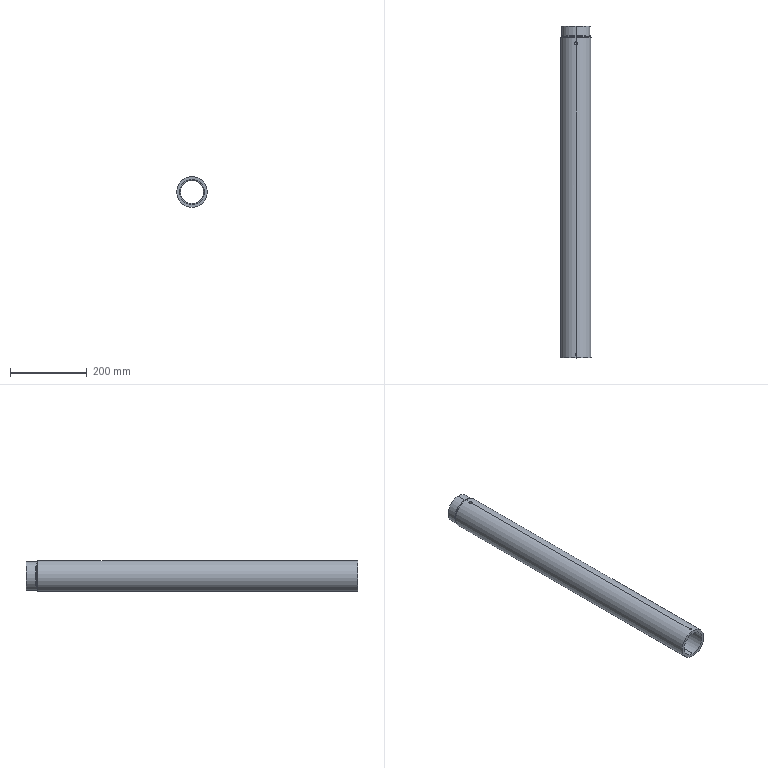Part | SolidWorks | features ICE 5, Chamfer 2, Extrusion 1, HoleWzd 1 | 1 solid | 24 faces | box 80 x 864.5 x 80 mm | volume 1857047 mm3 | cylinder 16 | plane 6 | cone 2 | commonest cylinder face diameters 4.2 x2 8 x2 60 x2 65 x2 73 x2 75 x2
STEP:
#1=CARTESIAN_POINT('',(0.,815.5,30.));
#2=VERTEX_POINT('',#1);
#3=CARTESIAN_POINT('',(-4.,819.5,29.732));
#4=VERTEX_POINT('',#3);
#5=CARTESIAN_POINT('',(0.,815.5,30.));
#6=CARTESIAN_POINT('',(-0.2612,815.5,30.));
#7=CARTESIAN_POINT('',(-0.5265,815.526,29.996));
#8=CARTESIAN_POINT('',(-1.04,815.629,29.983));
#9=CARTESIAN_POINT('',(-1.289,815.704,29.973));
#10=CARTESIAN_POINT('',(-1.773,815.905,29.949));
#11=CARTESIAN_POINT('',(-2.007,816.03,29.934));
#12=CARTESIAN_POINT('',(-2.44,816.32,29.901));
#13=CARTESIAN_POINT('',(-2.642,816.485,29.884));
#14=CARTESIAN_POINT('',(-3.015,816.858,29.849));
#15=CARTESIAN_POINT('',(-3.18,817.06,29.831));
#16=CARTESIAN_POINT('',(-3.47,817.493,29.799));
#17=CARTESIAN_POINT('',(-3.595,817.727,29.784));
#18=CARTESIAN_POINT('',(-3.796,818.211,29.759));
#19=CARTESIAN_POINT('',(-3.871,818.46,29.749));
#20=CARTESIAN_POINT('',(-3.974,818.974,29.736));
#21=CARTESIAN_POINT('',(-4.,819.239,29.732));
#22=CARTESIAN_POINT('',(-4.,819.5,29.732));
#23=B_SPLINE_CURVE_WITH_KNOTS('',3,(#5,#6,#7,#8,#9,#10,#11,#12,#13,#14,#15,#16,#17,#18,#19,#20,#21,#22),.UNSPECIFIED.,.F.,.F.,(4,2,2,2,2,2,2,2,4),(0.006261,0.007044,0.007826,0.008608,0.009391,0.01017,0.01096,0.01174,0.01252),.UNSPECIFIED.);
#24=EDGE_CURVE('',#2,#4,#23,.T.);
#25=ORIENTED_EDGE('',*,*,#24,.T.);
#26=CARTESIAN_POINT('',(-4.,819.5,39.799));
#27=VERTEX_POINT('',#26);
#28=CARTESIAN_POINT('',(-4.,819.5,10.));
#29=DIRECTION('',(0.,0.,1.));
#30=VECTOR('',#29,1000.);
#31=LINE('',#28,#30);
#32=EDGE_CURVE('',#4,#27,#31,.T.);
#33=ORIENTED_EDGE('',*,*,#32,.T.);
#34=CARTESIAN_POINT('',(0.,815.5,40.));
#35=VERTEX_POINT('',#34);
#36=CARTESIAN_POINT('',(0.,815.5,40.));
#37=CARTESIAN_POINT('',(-0.261,815.5,40.));
#38=CARTESIAN_POINT('',(-0.5262,815.526,39.997));
#39=CARTESIAN_POINT('',(-1.039,815.628,39.987));
#40=CARTESIAN_POINT('',(-1.289,815.704,39.98));
#41=CARTESIAN_POINT('',(-1.773,815.905,39.961));
#42=CARTESIAN_POINT('',(-2.007,816.03,39.95));
#43=CARTESIAN_POINT('',(-2.44,816.32,39.926));
#44=CARTESIAN_POINT('',(-2.642,816.485,39.913));
#45=CARTESIAN_POINT('',(-3.015,816.858,39.887));
#46=CARTESIAN_POINT('',(-3.181,817.06,39.874));
#47=CARTESIAN_POINT('',(-3.47,817.493,39.849));
#48=CARTESIAN_POINT('',(-3.595,817.727,39.838));
#49=CARTESIAN_POINT('',(-3.796,818.212,39.82));
#50=CARTESIAN_POINT('',(-3.872,818.461,39.812));
#51=CARTESIAN_POINT('',(-3.974,818.974,39.802));
#52=CARTESIAN_POINT('',(-4.,819.239,39.799));
#53=CARTESIAN_POINT('',(-4.,819.5,39.799));
#54=B_SPLINE_CURVE_WITH_KNOTS('',3,(#36,#37,#38,#39,#40,#41,#42,#43,#44,#45,#46,#47,#48,#49,#50,#51,#52,#53),.UNSPECIFIED.,.F.,.F.,(4,2,2,2,2,2,2,2,4),(0.006258,0.00704,0.007822,0.008604,0.009386,0.01017,0.01095,0.01173,0.01251),.UNSPECIFIED.);
#55=EDGE_CURVE('',#35,#27,#54,.T.);
#56=ORIENTED_EDGE('',*,*,#55,.F.);
#57=CARTESIAN_POINT('',(4.,819.5,39.799));
#58=VERTEX_POINT('',#57);
#59=CARTESIAN_POINT('',(4.,819.5,39.799));
#60=CARTESIAN_POINT('',(4.,819.235,39.799));
#61=CARTESIAN_POINT('',(3.974,818.975,39.802));
#62=CARTESIAN_POINT('',(3.872,818.464,39.812));
#63=CARTESIAN_POINT('',(3.795,818.21,39.82));
#64=CARTESIAN_POINT('',(3.594,817.725,39.838));
#65=CARTESIAN_POINT('',(3.471,817.495,39.849));
#66=CARTESIAN_POINT('',(3.181,817.061,39.874));
#67=CARTESIAN_POINT('',(3.012,816.855,39.887));
#68=CARTESIAN_POINT('',(2.643,816.486,39.913));
#69=CARTESIAN_POINT('',(2.441,816.321,39.926));
#70=CARTESIAN_POINT('',(2.004,816.028,39.95));
#71=CARTESIAN_POINT('',(1.771,815.904,39.961));
#72=CARTESIAN_POINT('',(1.29,815.705,39.98));
#73=CARTESIAN_POINT('',(1.037,815.628,39.987));
#74=CARTESIAN_POINT('',(0.5209,815.525,39.997));
#75=CARTESIAN_POINT('',(0.2611,815.5,40.));
#76=CARTESIAN_POINT('',(0.,815.5,40.));
#77=B_SPLINE_CURVE_WITH_KNOTS('',3,(#59,#60,#61,#62,#63,#64,#65,#66,#67,#68,#69,#70,#71,#72,#73,#74,#75,#76),.UNSPECIFIED.,.F.,.F.,(4,2,2,2,2,2,2,2,4),(0.,0.0007823,0.001565,0.002347,0.003129,0.003911,0.004694,0.005476,0.006258),.UNSPECIFIED.);
#78=EDGE_CURVE('',#58,#35,#77,.T.);
#79=ORIENTED_EDGE('',*,*,#78,.F.);
#80=CARTESIAN_POINT('',(4.,819.5,29.732));
#81=VERTEX_POINT('',#80);
#82=CARTESIAN_POINT('',(4.,819.5,10.));
#83=DIRECTION('',(0.,0.,1.));
#84=VECTOR('',#83,1000.);
#85=LINE('',#82,#84);
#86=EDGE_CURVE('',#81,#58,#85,.T.);
#87=ORIENTED_EDGE('',*,*,#86,.F.);
#88=CARTESIAN_POINT('',(4.,819.5,29.732));
#89=CARTESIAN_POINT('',(4.,819.235,29.732));
#90=CARTESIAN_POINT('',(3.974,818.975,29.736));
#91=CARTESIAN_POINT('',(3.872,818.463,29.749));
#92=CARTESIAN_POINT('',(3.795,818.209,29.759));
#93=CARTESIAN_POINT('',(3.594,817.725,29.784));
#94=CARTESIAN_POINT('',(3.471,817.495,29.799));
#95=CARTESIAN_POINT('',(3.181,817.06,29.831));
#96=CARTESIAN_POINT('',(3.012,816.855,29.849));
#97=CARTESIAN_POINT('',(2.643,816.486,29.884));
#98=CARTESIAN_POINT('',(2.442,816.321,29.901));
#99=CARTESIAN_POINT('',(2.004,816.028,29.934));
#100=CARTESIAN_POINT('',(1.772,815.904,29.949));
#101=CARTESIAN_POINT('',(1.29,815.705,29.973));
#102=CARTESIAN_POINT('',(1.038,815.628,29.983));
#103=CARTESIAN_POINT('',(0.5211,815.525,29.997));
#104=CARTESIAN_POINT('',(0.2613,815.5,30.));
#105=CARTESIAN_POINT('',(0.,815.5,30.));
#106=B_SPLINE_CURVE_WITH_KNOTS('',3,(#88,#89,#90,#91,#92,#93,#94,#95,#96,#97,#98,#99,#100,#101,#102,#103,#104,#105),.UNSPECIFIED.,.F.,.F.,(4,2,2,2,2,2,2,2,4),(0.,0.0007827,0.001565,0.002348,0.003131,0.003913,0.004696,0.005479,0.006261),.UNSPECIFIED.);
#107=EDGE_CURVE('',#81,#2,#106,.T.);
#108=ORIENTED_EDGE('',*,*,#107,.T.);
#109=EDGE_LOOP('',(#25,#33,#56,#79,#87,#108));
#110=FACE_OUTER_BOUND('',#109,.T.);
#111=CARTESIAN_POINT('',(0.,819.5,10.));
#112=DIRECTION('',(0.,0.,1.));
#113=DIRECTION('',(1.,0.,0.));
#114=AXIS2_PLACEMENT_3D('',#111,#112,#113);
#115=CYLINDRICAL_SURFACE('',#114,4.);
#116=ADVANCED_FACE('',(#110),#115,.F.);
#117=CARTESIAN_POINT('',(-2.1,9.,32.432));
#118=VERTEX_POINT('',#117);
#119=CARTESIAN_POINT('',(0.,6.9,32.5));
#120=VERTEX_POINT('',#119);
#121=CARTESIAN_POINT('',(-2.1,9.,32.432));
#122=CARTESIAN_POINT('',(-2.1,8.726,32.432));
#123=CARTESIAN_POINT('',(-2.045,8.449,32.436));
#124=CARTESIAN_POINT('',(-1.836,7.944,32.448));
#125=CARTESIAN_POINT('',(-1.679,7.709,32.457));
#126=CARTESIAN_POINT('',(-1.389,7.419,32.47));
#127=CARTESIAN_POINT('',(-1.281,7.33,32.475));
#128=CARTESIAN_POINT('',(-1.052,7.177,32.483));
#129=CARTESIAN_POINT('',(-0.9315,7.113,32.487));
#130=CARTESIAN_POINT('',(-0.6773,7.007,32.493));
#131=CARTESIAN_POINT('',(-0.5437,6.967,32.496));
#132=CARTESIAN_POINT('',(-0.2751,6.914,32.499));
#133=CARTESIAN_POINT('',(-0.1387,6.9,32.5));
#134=CARTESIAN_POINT('',(0.,6.9,32.5));
#135=B_SPLINE_CURVE_WITH_KNOTS('',3,(#121,#122,#123,#124,#125,#126,#127,#128,#129,#130,#131,#132,#133,#134),.UNSPECIFIED.,.F.,.F.,(4,2,2,2,2,2,4),(0.006567,0.007388,0.00821,0.00862,0.009031,0.009441,0.009852),.UNSPECIFIED.);
#136=EDGE_CURVE('',#118,#120,#135,.T.);
#137=ORIENTED_EDGE('',*,*,#136,.F.);
#138=CARTESIAN_POINT('',(-2.1,9.,39.945));
#139=VERTEX_POINT('',#138);
#140=CARTESIAN_POINT('',(-2.1,9.,40.));
#141=DIRECTION('',(0.,0.,1.));
#142=VECTOR('',#141,1000.);
#143=LINE('',#140,#142);
#144=EDGE_CURVE('',#118,#139,#143,.T.);
#145=ORIENTED_EDGE('',*,*,#144,.T.);
#146=CARTESIAN_POINT('',(0.,6.9,40.));
#147=VERTEX_POINT('',#146);
#148=CARTESIAN_POINT('',(0.,6.9,40.));
#149=CARTESIAN_POINT('',(-0.137,6.9,40.));
#150=CARTESIAN_POINT('',(-0.2761,6.914,39.999));
#151=CARTESIAN_POINT('',(-0.5454,6.967,39.997));
#152=CARTESIAN_POINT('',(-0.6762,7.007,39.994));
#153=CARTESIAN_POINT('',(-0.9305,7.112,39.989));
#154=CARTESIAN_POINT('',(-1.053,7.178,39.986));
#155=CARTESIAN_POINT('',(-1.281,7.33,39.98));
#156=CARTESIAN_POINT('',(-1.387,7.417,39.976));
#157=CARTESIAN_POINT('',(-1.583,7.613,39.969));
#158=CARTESIAN_POINT('',(-1.67,7.719,39.965));
#159=CARTESIAN_POINT('',(-1.822,7.947,39.959));
#160=CARTESIAN_POINT('',(-1.888,8.069,39.955));
#161=CARTESIAN_POINT('',(-1.993,8.324,39.95));
#162=CARTESIAN_POINT('',(-2.033,8.455,39.948));
#163=CARTESIAN_POINT('',(-2.086,8.724,39.946));
#164=CARTESIAN_POINT('',(-2.1,8.863,39.945));
#165=CARTESIAN_POINT('',(-2.1,9.,39.945));
#166=B_SPLINE_CURVE_WITH_KNOTS('',3,(#148,#149,#150,#151,#152,#153,#154,#155,#156,#157,#158,#159,#160,#161,#162,#163,#164,#165),.UNSPECIFIED.,.F.,.F.,(4,2,2,2,2,2,2,2,4),(0.003284,0.003694,0.004105,0.004515,0.004925,0.005336,0.005746,0.006156,0.006567),.UNSPECIFIED.);
#167=EDGE_CURVE('',#147,#139,#166,.T.);
#168=ORIENTED_EDGE('',*,*,#167,.F.);
#169=CARTESIAN_POINT('',(2.1,9.,39.945));
#170=VERTEX_POINT('',#169);
#171=CARTESIAN_POINT('',(2.1,9.,39.945));
#172=CARTESIAN_POINT('',(2.1,8.861,39.945));
#173=CARTESIAN_POINT('',(2.086,8.725,39.946));
#174=CARTESIAN_POINT('',(2.033,8.456,39.948));
#175=CARTESIAN_POINT('',(1.993,8.323,39.95));
#176=CARTESIAN_POINT('',(1.887,8.068,39.955));
#177=CARTESIAN_POINT('',(1.823,7.948,39.959));
#178=CARTESIAN_POINT('',(1.67,7.719,39.965));
#179=CARTESIAN_POINT('',(1.581,7.611,39.969));
#180=CARTESIAN_POINT('',(1.291,7.321,39.98));
#181=CARTESIAN_POINT('',(1.056,7.164,39.987));
#182=CARTESIAN_POINT('',(0.5506,6.955,39.997));
#183=CARTESIAN_POINT('',(0.2741,6.9,40.));
#184=CARTESIAN_POINT('',(0.,6.9,40.));
#185=B_SPLINE_CURVE_WITH_KNOTS('',3,(#171,#172,#173,#174,#175,#176,#177,#178,#179,#180,#181,#182,#183,#184),.UNSPECIFIED.,.F.,.F.,(4,2,2,2,2,2,4),(0.,0.0004105,0.000821,0.001232,0.001642,0.002463,0.003284),.UNSPECIFIED.);
#186=EDGE_CURVE('',#170,#147,#185,.T.);
#187=ORIENTED_EDGE('',*,*,#186,.F.);
#188=CARTESIAN_POINT('',(2.1,9.,32.432));
#189=VERTEX_POINT('',#188);
#190=CARTESIAN_POINT('',(2.1,9.,40.));
#191=DIRECTION('',(0.,0.,1.));
#192=VECTOR('',#191,1000.);
#193=LINE('',#190,#192);
#194=EDGE_CURVE('',#189,#170,#193,.T.);
#195=ORIENTED_EDGE('',*,*,#194,.F.);
#196=CARTESIAN_POINT('',(0.,6.9,32.5));
#197=CARTESIAN_POINT('',(0.1385,6.9,32.5));
#198=CARTESIAN_POINT('',(0.2753,6.914,32.499));
#199=CARTESIAN_POINT('',(0.5435,6.967,32.496));
#200=CARTESIAN_POINT('',(0.6766,7.007,32.493));
#201=CARTESIAN_POINT('',(0.931,7.113,32.487));
#202=CARTESIAN_POINT('',(1.052,7.177,32.483));
#203=CARTESIAN_POINT('',(1.28,7.329,32.475));
#204=CARTESIAN_POINT('',(1.388,7.418,32.471));
#205=CARTESIAN_POINT('',(1.581,7.611,32.462));
#206=CARTESIAN_POINT('',(1.668,7.717,32.457));
#207=CARTESIAN_POINT('',(1.822,7.946,32.449));
#208=CARTESIAN_POINT('',(1.887,8.068,32.445));
#209=CARTESIAN_POINT('',(2.044,8.447,32.436));
#210=CARTESIAN_POINT('',(2.1,8.723,32.432));
#211=CARTESIAN_POINT('',(2.1,9.,32.432));
#212=B_SPLINE_CURVE_WITH_KNOTS('',3,(#196,#197,#198,#199,#200,#201,#202,#203,#204,#205,#206,#207,#208,#209,#210,#211),.UNSPECIFIED.,.F.,.F.,(4,2,2,2,2,2,2,4),(0.009852,0.01026,0.01067,0.01108,0.01149,0.0119,0.01231,0.01313),.UNSPECIFIED.);
#213=EDGE_CURVE('',#120,#189,#212,.T.);
#214=ORIENTED_EDGE('',*,*,#213,.F.);
#215=EDGE_LOOP('',(#137,#145,#168,#187,#195,#214));
#216=FACE_OUTER_BOUND('',#215,.T.);
#217=CARTESIAN_POINT('',(0.,9.,40.));
#218=DIRECTION('',(0.,0.,1.));
#219=DIRECTION('',(1.,0.,0.));
#220=AXIS2_PLACEMENT_3D('',#217,#218,#219);
#221=CYLINDRICAL_SURFACE('',#220,2.1);
#222=ADVANCED_FACE('',(#216),#221,.F.);
#223=CARTESIAN_POINT('',(0.,51.5,30.));
#224=VERTEX_POINT('',#223);
#225=CARTESIAN_POINT('',(0.,51.5,-30.));
#226=VERTEX_POINT('',#225);
#227=CARTESIAN_POINT('',(0.,51.5,0.));
#228=DIRECTION('',(0.,-1.,0.));
#229=DIRECTION('',(0.,0.,-1.));
#230=AXIS2_PLACEMENT_3D('',#227,#228,#229);
#231=CIRCLE('',#230,30.);
#232=EDGE_CURVE('',#224,#226,#231,.T.);
#233=ORIENTED_EDGE('',*,*,#232,.F.);
#234=CARTESIAN_POINT('',(0.,50.,31.5));
#235=VERTEX_POINT('',#234);
#236=CARTESIAN_POINT('',(0.,51.5,30.));
#237=DIRECTION('',(0.,-0.7071,0.7071));
#238=VECTOR('',#237,1000.);
#239=LINE('',#236,#238);
#240=EDGE_CURVE('',#224,#235,#239,.T.);
#241=ORIENTED_EDGE('',*,*,#240,.T.);
#242=CARTESIAN_POINT('',(0.,50.,-31.5));
#243=VERTEX_POINT('',#242);
#244=CARTESIAN_POINT('',(0.,50.,0.));
#245=DIRECTION('',(0.,1.,0.));
#246=DIRECTION('',(0.,0.,-1.));
#247=AXIS2_PLACEMENT_3D('',#244,#245,#246);
#248=CIRCLE('',#247,31.5);
#249=EDGE_CURVE('',#243,#235,#248,.T.);
#250=ORIENTED_EDGE('',*,*,#249,.F.);
#251=CARTESIAN_POINT('',(0.,51.5,-30.));
#252=DIRECTION('',(0.,-0.7071,-0.7071));
#253=VECTOR('',#252,1000.);
#254=LINE('',#251,#253);
#255=EDGE_CURVE('',#226,#243,#254,.T.);
#256=ORIENTED_EDGE('',*,*,#255,.F.);
#257=EDGE_LOOP('',(#233,#241,#250,#256));
#258=FACE_OUTER_BOUND('',#257,.T.);
#259=CARTESIAN_POINT('',(0.,51.5,0.));
#260=DIRECTION('',(0.,-1.,0.));
#261=DIRECTION('',(0.,0.,-1.));
#262=AXIS2_PLACEMENT_3D('',#259,#260,#261);
#263=CONICAL_SURFACE('',#262,30.,0.7854);
#264=ADVANCED_FACE('',(#258),#263,.F.);
#265=CARTESIAN_POINT('',(0.,50.,32.5));
#266=VERTEX_POINT('',#265);
#267=CARTESIAN_POINT('',(0.,50.,-32.5));
#268=VERTEX_POINT('',#267);
#269=CARTESIAN_POINT('',(0.,50.,0.));
#270=DIRECTION('',(0.,-1.,0.));
#271=DIRECTION('',(0.,0.,-1.));
#272=AXIS2_PLACEMENT_3D('',#269,#270,#271);
#273=CIRCLE('',#272,32.5);
#274=EDGE_CURVE('',#266,#268,#273,.T.);
#275=ORIENTED_EDGE('',*,*,#274,.F.);
#276=CARTESIAN_POINT('',(0.,11.1,32.5));
#277=VERTEX_POINT('',#276);
#278=CARTESIAN_POINT('',(0.,50.,32.5));
#279=DIRECTION('',(0.,-1.,0.));
#280=VECTOR('',#279,1000.);
#281=LINE('',#278,#280);
#282=EDGE_CURVE('',#266,#277,#281,.T.);
#283=ORIENTED_EDGE('',*,*,#282,.T.);
#284=CARTESIAN_POINT('',(0.,11.1,32.5));
#285=CARTESIAN_POINT('',(-0.137,11.1,32.5));
#286=CARTESIAN_POINT('',(-0.2761,11.086,32.499));
#287=CARTESIAN_POINT('',(-0.5454,11.033,32.496));
#288=CARTESIAN_POINT('',(-0.6763,10.993,32.493));
#289=CARTESIAN_POINT('',(-0.9305,10.888,32.487));
#290=CARTESIAN_POINT('',(-1.053,10.822,32.483));
#291=CARTESIAN_POINT('',(-1.281,10.67,32.475));
#292=CARTESIAN_POINT('',(-1.387,10.583,32.471));
#293=CARTESIAN_POINT('',(-1.583,10.387,32.462));
#294=CARTESIAN_POINT('',(-1.67,10.281,32.457));
#295=CARTESIAN_POINT('',(-1.822,10.053,32.449));
#296=CARTESIAN_POINT('',(-1.888,9.931,32.445));
#297=CARTESIAN_POINT('',(-1.993,9.676,32.439));
#298=CARTESIAN_POINT('',(-2.033,9.545,32.436));
#299=CARTESIAN_POINT('',(-2.086,9.276,32.433));
#300=CARTESIAN_POINT('',(-2.1,9.137,32.432));
#301=CARTESIAN_POINT('',(-2.1,9.,32.432));
#302=B_SPLINE_CURVE_WITH_KNOTS('',3,(#284,#285,#286,#287,#288,#289,#290,#291,#292,#293,#294,#295,#296,#297,#298,#299,#300,#301),.UNSPECIFIED.,.F.,.F.,(4,2,2,2,2,2,2,2,4),(0.003284,0.003695,0.004105,0.004515,0.004926,0.005336,0.005747,0.006157,0.006567),.UNSPECIFIED.);
#303=EDGE_CURVE('',#277,#118,#302,.T.);
#304=ORIENTED_EDGE('',*,*,#303,.T.);
#305=ORIENTED_EDGE('',*,*,#136,.T.);
#306=CARTESIAN_POINT('',(0.,0.,32.5));
#307=VERTEX_POINT('',#306);
#308=CARTESIAN_POINT('',(0.,50.,32.5));
#309=DIRECTION('',(0.,-1.,0.));
#310=VECTOR('',#309,1000.);
#311=LINE('',#308,#310);
#312=EDGE_CURVE('',#120,#307,#311,.T.);
#313=ORIENTED_EDGE('',*,*,#312,.T.);
#314=CARTESIAN_POINT('',(0.,0.,-32.5));
#315=VERTEX_POINT('',#314);
#316=CARTESIAN_POINT('',(0.,0.,0.));
#317=DIRECTION('',(0.,-1.,0.));
#318=DIRECTION('',(0.,0.,-1.));
#319=AXIS2_PLACEMENT_3D('',#316,#317,#318);
#320=CIRCLE('',#319,32.5);
#321=EDGE_CURVE('',#307,#315,#320,.T.);
#322=ORIENTED_EDGE('',*,*,#321,.T.);
#323=CARTESIAN_POINT('',(0.,50.,-32.5));
#324=DIRECTION('',(0.,-1.,0.));
#325=VECTOR('',#324,1000.);
#326=LINE('',#323,#325);
#327=EDGE_CURVE('',#268,#315,#326,.T.);
#328=ORIENTED_EDGE('',*,*,#327,.F.);
#329=EDGE_LOOP('',(#275,#283,#304,#305,#313,#322,#328));
#330=FACE_OUTER_BOUND('',#329,.T.);
#331=CARTESIAN_POINT('',(0.,50.,0.));
#332=DIRECTION('',(0.,-1.,0.));
#333=DIRECTION('',(0.,0.,-1.));
#334=AXIS2_PLACEMENT_3D('',#331,#332,#333);
#335=CYLINDRICAL_SURFACE('',#334,32.5);
#336=ADVANCED_FACE('',(#330),#335,.F.);
#337=CARTESIAN_POINT('',(0.,834.5,38.));
#338=VERTEX_POINT('',#337);
#339=CARTESIAN_POINT('',(0.,834.5,-38.));
#340=VERTEX_POINT('',#339);
#341=CARTESIAN_POINT('',(0.,834.5,0.));
#342=DIRECTION('',(0.,1.,0.));
#343=DIRECTION('',(0.,0.,1.));
#344=AXIS2_PLACEMENT_3D('',#341,#342,#343);
#345=CIRCLE('',#344,38.);
#346=EDGE_CURVE('',#338,#340,#345,.T.);
#347=ORIENTED_EDGE('',*,*,#346,.T.);
#348=CARTESIAN_POINT('',(0.,836.5,-38.));
#349=VERTEX_POINT('',#348);
#350=CARTESIAN_POINT('',(0.,834.5,-38.));
#351=DIRECTION('',(0.,1.,0.));
#352=VECTOR('',#351,1000.);
#353=LINE('',#350,#352);
#354=EDGE_CURVE('',#340,#349,#353,.T.);
#355=ORIENTED_EDGE('',*,*,#354,.T.);
#356=CARTESIAN_POINT('',(0.,836.5,38.));
#357=VERTEX_POINT('',#356);
#358=CARTESIAN_POINT('',(0.,836.5,0.));
#359=DIRECTION('',(0.,1.,0.));
#360=DIRECTION('',(0.,0.,1.));
#361=AXIS2_PLACEMENT_3D('',#358,#359,#360);
#362=CIRCLE('',#361,38.);
#363=EDGE_CURVE('',#357,#349,#362,.T.);
#364=ORIENTED_EDGE('',*,*,#363,.F.);
#365=CARTESIAN_POINT('',(0.,834.5,38.));
#366=DIRECTION('',(0.,1.,0.));
#367=VECTOR('',#366,1000.);
#368=LINE('',#365,#367);
#369=EDGE_CURVE('',#338,#357,#368,.T.);
#370=ORIENTED_EDGE('',*,*,#369,.F.);
#371=EDGE_LOOP('',(#347,#355,#364,#370));
#372=FACE_OUTER_BOUND('',#371,.T.);
#373=CARTESIAN_POINT('',(0.,834.5,0.));
#374=DIRECTION('',(0.,1.,0.));
#375=DIRECTION('',(0.,0.,1.));
#376=AXIS2_PLACEMENT_3D('',#373,#374,#375);
#377=CYLINDRICAL_SURFACE('',#376,38.);
#378=ADVANCED_FACE('',(#372),#377,.T.);
#379=CARTESIAN_POINT('',(0.,836.5,36.5));
#380=VERTEX_POINT('',#379);
#381=CARTESIAN_POINT('',(0.,836.5,-36.5));
#382=VERTEX_POINT('',#381);
#383=CARTESIAN_POINT('',(0.,836.5,0.));
#384=DIRECTION('',(0.,1.,0.));
#385=DIRECTION('',(0.,0.,1.));
#386=AXIS2_PLACEMENT_3D('',#383,#384,#385);
#387=CIRCLE('',#386,36.5);
#388=EDGE_CURVE('',#380,#382,#387,.T.);
#389=ORIENTED_EDGE('',*,*,#388,.T.);
#390=CARTESIAN_POINT('',(0.,839.5,-36.5));
#391=VERTEX_POINT('',#390);
#392=CARTESIAN_POINT('',(0.,836.5,-36.5));
#393=DIRECTION('',(0.,1.,0.));
#394=VECTOR('',#393,1000.);
#395=LINE('',#392,#394);
#396=EDGE_CURVE('',#382,#391,#395,.T.);
#397=ORIENTED_EDGE('',*,*,#396,.T.);
#398=CARTESIAN_POINT('',(0.,839.5,36.5));
#399=VERTEX_POINT('',#398);
#400=CARTESIAN_POINT('',(0.,839.5,0.));
#401=DIRECTION('',(0.,1.,0.));
#402=DIRECTION('',(0.,0.,1.));
#403=AXIS2_PLACEMENT_3D('',#400,#401,#402);
#404=CIRCLE('',#403,36.5);
#405=EDGE_CURVE('',#399,#391,#404,.T.);
#406=ORIENTED_EDGE('',*,*,#405,.F.);
#407=CARTESIAN_POINT('',(0.,836.5,36.5));
#408=DIRECTION('',(0.,1.,0.));
#409=VECTOR('',#408,1000.);
#410=LINE('',#407,#409);
#411=EDGE_CURVE('',#380,#399,#410,.T.);
#412=ORIENTED_EDGE('',*,*,#411,.F.);
#413=EDGE_LOOP('',(#389,#397,#406,#412));
#414=FACE_OUTER_BOUND('',#413,.T.);
#415=CARTESIAN_POINT('',(0.,836.5,0.));
#416=DIRECTION('',(0.,1.,0.));
#417=DIRECTION('',(0.,0.,1.));
#418=AXIS2_PLACEMENT_3D('',#415,#416,#417);
#419=CYLINDRICAL_SURFACE('',#418,36.5);
#420=ADVANCED_FACE('',(#414),#419,.T.);
#421=CARTESIAN_POINT('',(0.,839.5,-37.5));
#422=VERTEX_POINT('',#421);
#423=CARTESIAN_POINT('',(0.,839.5,37.5));
#424=VERTEX_POINT('',#423);
#425=CARTESIAN_POINT('',(0.,839.5,0.));
#426=DIRECTION('',(0.,-1.,0.));
#427=DIRECTION('',(0.,0.,1.));
#428=AXIS2_PLACEMENT_3D('',#425,#426,#427);
#429=CIRCLE('',#428,37.5);
#430=EDGE_CURVE('',#422,#424,#429,.T.);
#431=ORIENTED_EDGE('',*,*,#430,.F.);
#432=CARTESIAN_POINT('',(0.,864.5,-37.5));
#433=VERTEX_POINT('',#432);
#434=CARTESIAN_POINT('',(0.,839.5,-37.5));
#435=DIRECTION('',(0.,1.,0.));
#436=VECTOR('',#435,1000.);
#437=LINE('',#434,#436);
#438=EDGE_CURVE('',#422,#433,#437,.T.);
#439=ORIENTED_EDGE('',*,*,#438,.T.);
#440=CARTESIAN_POINT('',(0.,864.5,37.5));
#441=VERTEX_POINT('',#440);
#442=CARTESIAN_POINT('',(0.,864.5,0.));
#443=DIRECTION('',(0.,1.,0.));
#444=DIRECTION('',(0.,0.,1.));
#445=AXIS2_PLACEMENT_3D('',#442,#443,#444);
#446=CIRCLE('',#445,37.5);
#447=EDGE_CURVE('',#441,#433,#446,.T.);
#448=ORIENTED_EDGE('',*,*,#447,.F.);
#449=CARTESIAN_POINT('',(0.,839.5,37.5));
#450=DIRECTION('',(0.,1.,0.));
#451=VECTOR('',#450,1000.);
#452=LINE('',#449,#451);
#453=EDGE_CURVE('',#424,#441,#452,.T.);
#454=ORIENTED_EDGE('',*,*,#453,.F.);
#455=EDGE_LOOP('',(#431,#439,#448,#454));
#456=FACE_OUTER_BOUND('',#455,.T.);
#457=CARTESIAN_POINT('',(0.,839.5,0.));
#458=DIRECTION('',(0.,1.,0.));
#459=DIRECTION('',(0.,0.,1.));
#460=AXIS2_PLACEMENT_3D('',#457,#458,#459);
#461=CYLINDRICAL_SURFACE('',#460,37.5);
#462=ADVANCED_FACE('',(#456),#461,.T.);
#463=CARTESIAN_POINT('',(0.,834.5,40.));
#464=VERTEX_POINT('',#463);
#465=CARTESIAN_POINT('',(0.,834.5,-40.));
#466=VERTEX_POINT('',#465);
#467=CARTESIAN_POINT('',(0.,834.5,0.));
#468=DIRECTION('',(0.,1.,0.));
#469=DIRECTION('',(0.,0.,1.));
#470=AXIS2_PLACEMENT_3D('',#467,#468,#469);
#471=CIRCLE('',#470,40.);
#472=EDGE_CURVE('',#464,#466,#471,.T.);
#473=ORIENTED_EDGE('',*,*,#472,.F.);
#474=CARTESIAN_POINT('',(0.,823.5,40.));
#475=VERTEX_POINT('',#474);
#476=CARTESIAN_POINT('',(0.,864.5,40.));
#477=DIRECTION('',(0.,-1.,0.));
#478=VECTOR('',#477,1000.);
#479=LINE('',#476,#478);
#480=EDGE_CURVE('',#464,#475,#479,.T.);
#481=ORIENTED_EDGE('',*,*,#480,.T.);
#482=CARTESIAN_POINT('',(0.,823.5,40.));
#483=CARTESIAN_POINT('',(0.2641,823.5,40.));
#484=CARTESIAN_POINT('',(0.5243,823.474,39.997));
#485=CARTESIAN_POINT('',(1.035,823.372,39.987));
#486=CARTESIAN_POINT('',(1.289,823.296,39.98));
#487=CARTESIAN_POINT('',(1.774,823.095,39.961));
#488=CARTESIAN_POINT('',(2.003,822.972,39.95));
#489=CARTESIAN_POINT('',(2.438,822.682,39.926));
#490=CARTESIAN_POINT('',(2.643,822.514,39.913));
#491=CARTESIAN_POINT('',(3.012,822.145,39.887));
#492=CARTESIAN_POINT('',(3.177,821.944,39.874));
#493=CARTESIAN_POINT('',(3.47,821.507,39.849));
#494=CARTESIAN_POINT('',(3.594,821.275,39.838));
#495=CARTESIAN_POINT('',(3.794,820.794,39.82));
#496=CARTESIAN_POINT('',(3.871,820.543,39.812));
#497=CARTESIAN_POINT('',(3.974,820.026,39.802));
#498=CARTESIAN_POINT('',(4.,819.764,39.799));
#499=CARTESIAN_POINT('',(4.,819.5,39.799));
#500=B_SPLINE_CURVE_WITH_KNOTS('',3,(#482,#483,#484,#485,#486,#487,#488,#489,#490,#491,#492,#493,#494,#495,#496,#497,#498,#499),.UNSPECIFIED.,.F.,.F.,(4,2,2,2,2,2,2,2,4),(0.01877,0.01955,0.02034,0.02112,0.0219,0.02268,0.02346,0.02424,0.02502),.UNSPECIFIED.);
#501=EDGE_CURVE('',#475,#58,#500,.T.);
#502=ORIENTED_EDGE('',*,*,#501,.T.);
#503=ORIENTED_EDGE('',*,*,#78,.T.);
#504=CARTESIAN_POINT('',(0.,11.1,40.));
#505=VERTEX_POINT('',#504);
#506=CARTESIAN_POINT('',(0.,864.5,40.));
#507=DIRECTION('',(0.,-1.,0.));
#508=VECTOR('',#507,1000.);
#509=LINE('',#506,#508);
#510=EDGE_CURVE('',#35,#505,#509,.T.);
#511=ORIENTED_EDGE('',*,*,#510,.T.);
#512=CARTESIAN_POINT('',(0.,11.1,40.));
#513=CARTESIAN_POINT('',(0.1385,11.1,40.));
#514=CARTESIAN_POINT('',(0.2753,11.086,39.999));
#515=CARTESIAN_POINT('',(0.5435,11.033,39.997));
#516=CARTESIAN_POINT('',(0.6766,10.993,39.994));
#517=CARTESIAN_POINT('',(0.931,10.887,39.989));
#518=CARTESIAN_POINT('',(1.052,10.823,39.986));
#519=CARTESIAN_POINT('',(1.28,10.671,39.98));
#520=CARTESIAN_POINT('',(1.388,10.582,39.976));
#521=CARTESIAN_POINT('',(1.581,10.389,39.969));
#522=CARTESIAN_POINT('',(1.668,10.283,39.965));
#523=CARTESIAN_POINT('',(1.822,10.054,39.959));
#524=CARTESIAN_POINT('',(1.887,9.932,39.955));
#525=CARTESIAN_POINT('',(2.044,9.553,39.948));
#526=CARTESIAN_POINT('',(2.1,9.277,39.945));
#527=CARTESIAN_POINT('',(2.1,9.,39.945));
#528=B_SPLINE_CURVE_WITH_KNOTS('',3,(#512,#513,#514,#515,#516,#517,#518,#519,#520,#521,#522,#523,#524,#525,#526,#527),.UNSPECIFIED.,.F.,.F.,(4,2,2,2,2,2,2,4),(0.009851,0.01026,0.01067,0.01108,0.01149,0.0119,0.01231,0.01313),.UNSPECIFIED.);
#529=EDGE_CURVE('',#505,#170,#528,.T.);
#530=ORIENTED_EDGE('',*,*,#529,.T.);
#531=ORIENTED_EDGE('',*,*,#186,.T.);
#532=CARTESIAN_POINT('',(0.,0.,40.));
#533=VERTEX_POINT('',#532);
#534=CARTESIAN_POINT('',(0.,864.5,40.));
#535=DIRECTION('',(0.,-1.,0.));
#536=VECTOR('',#535,1000.);
#537=LINE('',#534,#536);
#538=EDGE_CURVE('',#147,#533,#537,.T.);
#539=ORIENTED_EDGE('',*,*,#538,.T.);
#540=CARTESIAN_POINT('',(0.,0.,-40.));
#541=VERTEX_POINT('',#540);
#542=CARTESIAN_POINT('',(0.,0.,0.));
#543=DIRECTION('',(0.,1.,0.));
#544=DIRECTION('',(0.,0.,1.));
#545=AXIS2_PLACEMENT_3D('',#542,#543,#544);
#546=CIRCLE('',#545,40.);
#547=EDGE_CURVE('',#533,#541,#546,.T.);
#548=ORIENTED_EDGE('',*,*,#547,.T.);
#549=CARTESIAN_POINT('',(0.,864.5,-40.));
#550=DIRECTION('',(0.,-1.,0.));
#551=VECTOR('',#550,1000.);
#552=LINE('',#549,#551);
#553=EDGE_CURVE('',#466,#541,#552,.T.);
#554=ORIENTED_EDGE('',*,*,#553,.F.);
#555=EDGE_LOOP('',(#473,#481,#502,#503,#511,#530,#531,#539,#548,#554));
#556=FACE_OUTER_BOUND('',#555,.T.);
#557=CARTESIAN_POINT('',(0.,864.5,0.));
#558=DIRECTION('',(0.,-1.,0.));
#559=DIRECTION('',(0.,0.,-1.));
#560=AXIS2_PLACEMENT_3D('',#557,#558,#559);
#561=CYLINDRICAL_SURFACE('',#560,40.);
#562=ADVANCED_FACE('',(#556),#561,.T.);
#563=CARTESIAN_POINT('',(0.,864.5,-30.));
#564=VERTEX_POINT('',#563);
#565=CARTESIAN_POINT('',(0.,864.5,30.));
#566=VERTEX_POINT('',#565);
#567=CARTESIAN_POINT('',(0.,864.5,0.));
#568=DIRECTION('',(0.,1.,0.));
#569=DIRECTION('',(0.,0.,1.));
#570=AXIS2_PLACEMENT_3D('',#567,#568,#569);
#571=CIRCLE('',#570,30.);
#572=EDGE_CURVE('',#564,#566,#571,.T.);
#573=ORIENTED_EDGE('',*,*,#572,.T.);
#574=CARTESIAN_POINT('',(0.,823.5,30.));
#575=VERTEX_POINT('',#574);
#576=CARTESIAN_POINT('',(0.,864.5,30.));
#577=DIRECTION('',(0.,-1.,0.));
#578=VECTOR('',#577,1000.);
#579=LINE('',#576,#578);
#580=EDGE_CURVE('',#566,#575,#579,.T.);
#581=ORIENTED_EDGE('',*,*,#580,.T.);
#582=CARTESIAN_POINT('',(-4.,819.5,29.732));
#583=CARTESIAN_POINT('',(-4.,819.761,29.732));
#584=CARTESIAN_POINT('',(-3.975,820.021,29.736));
#585=CARTESIAN_POINT('',(-3.872,820.538,29.749));
#586=CARTESIAN_POINT('',(-3.795,820.79,29.759));
#587=CARTESIAN_POINT('',(-3.596,821.272,29.784));
#588=CARTESIAN_POINT('',(-3.471,821.505,29.799));
#589=CARTESIAN_POINT('',(-3.179,821.942,29.831));
#590=CARTESIAN_POINT('',(-3.014,822.143,29.849));
#591=CARTESIAN_POINT('',(-2.645,822.512,29.884));
#592=CARTESIAN_POINT('',(-2.439,822.681,29.901));
#593=CARTESIAN_POINT('',(-2.005,822.971,29.934));
#594=CARTESIAN_POINT('',(-1.775,823.094,29.948));
#595=CARTESIAN_POINT('',(-1.291,823.295,29.973));
#596=CARTESIAN_POINT('',(-1.037,823.372,29.983));
#597=CARTESIAN_POINT('',(-0.525,823.474,29.996));
#598=CARTESIAN_POINT('',(-0.2645,823.5,30.));
#599=CARTESIAN_POINT('',(0.,823.5,30.));
#600=B_SPLINE_CURVE_WITH_KNOTS('',3,(#582,#583,#584,#585,#586,#587,#588,#589,#590,#591,#592,#593,#594,#595,#596,#597,#598,#599),.UNSPECIFIED.,.F.,.F.,(4,2,2,2,2,2,2,2,4),(0.01252,0.0133,0.01409,0.01487,0.01565,0.01643,0.01722,0.018,0.01878),.UNSPECIFIED.);
#601=EDGE_CURVE('',#4,#575,#600,.T.);
#602=ORIENTED_EDGE('',*,*,#601,.F.);
#603=ORIENTED_EDGE('',*,*,#24,.F.);
#604=CARTESIAN_POINT('',(0.,864.5,30.));
#605=DIRECTION('',(0.,-1.,0.));
#606=VECTOR('',#605,1000.);
#607=LINE('',#604,#606);
#608=EDGE_CURVE('',#2,#224,#607,.T.);
#609=ORIENTED_EDGE('',*,*,#608,.T.);
#610=ORIENTED_EDGE('',*,*,#232,.T.);
#611=CARTESIAN_POINT('',(0.,864.5,-30.));
#612=DIRECTION('',(0.,-1.,0.));
#613=VECTOR('',#612,1000.);
#614=LINE('',#611,#613);
#615=EDGE_CURVE('',#564,#226,#614,.T.);
#616=ORIENTED_EDGE('',*,*,#615,.F.);
#617=EDGE_LOOP('',(#573,#581,#602,#603,#609,#610,#616));
#618=FACE_OUTER_BOUND('',#617,.T.);
#619=CARTESIAN_POINT('',(0.,864.5,0.));
#620=DIRECTION('',(0.,-1.,0.));
#621=DIRECTION('',(0.,0.,-1.));
#622=AXIS2_PLACEMENT_3D('',#619,#620,#621);
#623=CYLINDRICAL_SURFACE('',#622,30.);
#624=ADVANCED_FACE('',(#618),#623,.F.);
#625=ORIENTED_EDGE('',*,*,#580,.F.);
#626=CARTESIAN_POINT('',(0.,864.5,0.));
#627=DIRECTION('',(0.,1.,0.));
#628=DIRECTION('',(0.,0.,1.));
#629=AXIS2_PLACEMENT_3D('',#626,#627,#628);
#630=CIRCLE('',#629,30.);
#631=EDGE_CURVE('',#566,#564,#630,.T.);
#632=ORIENTED_EDGE('',*,*,#631,.T.);
#633=ORIENTED_EDGE('',*,*,#615,.T.);
#634=CARTESIAN_POINT('',(0.,51.5,0.));
#635=DIRECTION('',(0.,-1.,0.));
#636=DIRECTION('',(0.,0.,-1.));
#637=AXIS2_PLACEMENT_3D('',#634,#635,#636);
#638=CIRCLE('',#637,30.);
#639=EDGE_CURVE('',#226,#224,#638,.T.);
#640=ORIENTED_EDGE('',*,*,#639,.T.);
#641=ORIENTED_EDGE('',*,*,#608,.F.);
#642=ORIENTED_EDGE('',*,*,#107,.F.);
#643=CARTESIAN_POINT('',(0.,823.5,30.));
#644=CARTESIAN_POINT('',(0.2643,823.5,30.));
#645=CARTESIAN_POINT('',(0.5242,823.474,29.997));
#646=CARTESIAN_POINT('',(1.036,823.372,29.983));
#647=CARTESIAN_POINT('',(1.29,823.295,29.973));
#648=CARTESIAN_POINT('',(1.774,823.095,29.949));
#649=CARTESIAN_POINT('',(2.003,822.972,29.934));
#650=CARTESIAN_POINT('',(2.438,822.682,29.902));
#651=CARTESIAN_POINT('',(2.643,822.513,29.884));
#652=CARTESIAN_POINT('',(3.012,822.145,29.849));
#653=CARTESIAN_POINT('',(3.177,821.944,29.832));
#654=CARTESIAN_POINT('',(3.47,821.507,29.799));
#655=CARTESIAN_POINT('',(3.594,821.275,29.784));
#656=CARTESIAN_POINT('',(3.794,820.795,29.759));
#657=CARTESIAN_POINT('',(3.871,820.543,29.749));
#658=CARTESIAN_POINT('',(3.974,820.026,29.736));
#659=CARTESIAN_POINT('',(4.,819.764,29.732));
#660=CARTESIAN_POINT('',(4.,819.5,29.732));
#661=B_SPLINE_CURVE_WITH_KNOTS('',3,(#643,#644,#645,#646,#647,#648,#649,#650,#651,#652,#653,#654,#655,#656,#657,#658,#659,#660),.UNSPECIFIED.,.F.,.F.,(4,2,2,2,2,2,2,2,4),(0.01878,0.01956,0.02034,0.02113,0.02191,0.02269,0.02347,0.02425,0.02504),.UNSPECIFIED.);
#662=EDGE_CURVE('',#575,#81,#661,.T.);
#663=ORIENTED_EDGE('',*,*,#662,.F.);
#664=EDGE_LOOP('',(#625,#632,#633,#640,#641,#642,#663));
#665=FACE_OUTER_BOUND('',#664,.T.);
#666=CARTESIAN_POINT('',(0.,864.5,0.));
#667=DIRECTION('',(0.,-1.,0.));
#668=DIRECTION('',(0.,0.,-1.));
#669=AXIS2_PLACEMENT_3D('',#666,#667,#668);
#670=CYLINDRICAL_SURFACE('',#669,30.);
#671=ADVANCED_FACE('',(#665),#670,.F.);
#672=ORIENTED_EDGE('',*,*,#480,.F.);
#673=CARTESIAN_POINT('',(0.,834.5,0.));
#674=DIRECTION('',(0.,1.,0.));
#675=DIRECTION('',(0.,0.,1.));
#676=AXIS2_PLACEMENT_3D('',#673,#674,#675);
#677=CIRCLE('',#676,40.);
#678=EDGE_CURVE('',#466,#464,#677,.T.);
#679=ORIENTED_EDGE('',*,*,#678,.F.);
#680=ORIENTED_EDGE('',*,*,#553,.T.);
#681=CARTESIAN_POINT('',(0.,0.,0.));
#682=DIRECTION('',(0.,1.,0.));
#683=DIRECTION('',(0.,0.,1.));
#684=AXIS2_PLACEMENT_3D('',#681,#682,#683);
#685=CIRCLE('',#684,40.);
#686=EDGE_CURVE('',#541,#533,#685,.T.);
#687=ORIENTED_EDGE('',*,*,#686,.T.);
#688=ORIENTED_EDGE('',*,*,#538,.F.);
#689=ORIENTED_EDGE('',*,*,#167,.T.);
#690=CARTESIAN_POINT('',(-2.1,9.,39.945));
#691=CARTESIAN_POINT('',(-2.1,9.137,39.945));
#692=CARTESIAN_POINT('',(-2.087,9.273,39.946));
#693=CARTESIAN_POINT('',(-2.033,9.544,39.948));
#694=CARTESIAN_POINT('',(-1.993,9.677,39.95));
#695=CARTESIAN_POINT('',(-1.836,10.056,39.958));
#696=CARTESIAN_POINT('',(-1.679,10.291,39.965));
#697=CARTESIAN_POINT('',(-1.389,10.581,39.976));
#698=CARTESIAN_POINT('',(-1.281,10.67,39.98));
#699=CARTESIAN_POINT('',(-1.052,10.823,39.986));
#700=CARTESIAN_POINT('',(-0.9314,10.887,39.989));
#701=CARTESIAN_POINT('',(-0.6772,10.993,39.994));
#702=CARTESIAN_POINT('',(-0.5436,11.033,39.997));
#703=CARTESIAN_POINT('',(-0.275,11.086,39.999));
#704=CARTESIAN_POINT('',(-0.1386,11.1,40.));
#705=CARTESIAN_POINT('',(0.,11.1,40.));
#706=B_SPLINE_CURVE_WITH_KNOTS('',3,(#690,#691,#692,#693,#694,#695,#696,#697,#698,#699,#700,#701,#702,#703,#704,#705),.UNSPECIFIED.,.F.,.F.,(4,2,2,2,2,2,2,4),(0.006567,0.006977,0.007388,0.008209,0.008619,0.00903,0.00944,0.009851),.UNSPECIFIED.);
#707=EDGE_CURVE('',#139,#505,#706,.T.);
#708=ORIENTED_EDGE('',*,*,#707,.T.);
#709=ORIENTED_EDGE('',*,*,#510,.F.);
#710=ORIENTED_EDGE('',*,*,#55,.T.);
#711=CARTESIAN_POINT('',(-4.,819.5,39.799));
#712=CARTESIAN_POINT('',(-4.,819.761,39.799));
#713=CARTESIAN_POINT('',(-3.975,820.021,39.802));
#714=CARTESIAN_POINT('',(-3.872,820.537,39.812));
#715=CARTESIAN_POINT('',(-3.795,820.79,39.82));
#716=CARTESIAN_POINT('',(-3.596,821.272,39.838));
#717=CARTESIAN_POINT('',(-3.472,821.504,39.849));
#718=CARTESIAN_POINT('',(-3.179,821.942,39.874));
#719=CARTESIAN_POINT('',(-3.014,822.143,39.887));
#720=CARTESIAN_POINT('',(-2.645,822.512,39.913));
#721=CARTESIAN_POINT('',(-2.439,822.681,39.926));
#722=CARTESIAN_POINT('',(-2.004,822.971,39.95));
#723=CARTESIAN_POINT('',(-1.775,823.094,39.961));
#724=CARTESIAN_POINT('',(-1.29,823.295,39.98));
#725=CARTESIAN_POINT('',(-1.036,823.372,39.987));
#726=CARTESIAN_POINT('',(-0.5244,823.474,39.997));
#727=CARTESIAN_POINT('',(-0.2644,823.5,40.));
#728=CARTESIAN_POINT('',(0.,823.5,40.));
#729=B_SPLINE_CURVE_WITH_KNOTS('',3,(#711,#712,#713,#714,#715,#716,#717,#718,#719,#720,#721,#722,#723,#724,#725,#726,#727,#728),.UNSPECIFIED.,.F.,.F.,(4,2,2,2,2,2,2,2,4),(0.01251,0.0133,0.01408,0.01486,0.01564,0.01643,0.01721,0.01799,0.01877),.UNSPECIFIED.);
#730=EDGE_CURVE('',#27,#475,#729,.T.);
#731=ORIENTED_EDGE('',*,*,#730,.T.);
#732=EDGE_LOOP('',(#672,#679,#680,#687,#688,#689,#708,#709,#710,#731));
#733=FACE_OUTER_BOUND('',#732,.T.);
#734=CARTESIAN_POINT('',(0.,864.5,0.));
#735=DIRECTION('',(0.,-1.,0.));
#736=DIRECTION('',(0.,0.,-1.));
#737=AXIS2_PLACEMENT_3D('',#734,#735,#736);
#738=CYLINDRICAL_SURFACE('',#737,40.);
#739=ADVANCED_FACE('',(#733),#738,.T.);
#740=ORIENTED_EDGE('',*,*,#388,.F.);
#741=CARTESIAN_POINT('',(0.,836.5,0.));
#742=DIRECTION('',(0.,1.,0.));
#743=DIRECTION('',(0.,0.,1.));
#744=AXIS2_PLACEMENT_3D('',#741,#742,#743);
#745=CIRCLE('',#744,36.5);
#746=EDGE_CURVE('',#382,#380,#745,.T.);
#747=ORIENTED_EDGE('',*,*,#746,.F.);
#748=EDGE_LOOP('',(#740,#747));
#749=FACE_BOUND('',#748,.T.);
#750=ORIENTED_EDGE('',*,*,#363,.T.);
#751=CARTESIAN_POINT('',(0.,836.5,0.));
#752=DIRECTION('',(0.,1.,0.));
#753=DIRECTION('',(0.,0.,1.));
#754=AXIS2_PLACEMENT_3D('',#751,#752,#753);
#755=CIRCLE('',#754,38.);
#756=EDGE_CURVE('',#349,#357,#755,.T.);
#757=ORIENTED_EDGE('',*,*,#756,.T.);
#758=EDGE_LOOP('',(#750,#757));
#759=FACE_OUTER_BOUND('',#758,.T.);
#760=CARTESIAN_POINT('',(0.,836.5,0.));
#761=DIRECTION('',(0.,1.,0.));
#762=DIRECTION('',(0.,0.,1.));
#763=AXIS2_PLACEMENT_3D('',#760,#761,#762);
#764=PLANE('',#763);
#765=ADVANCED_FACE('',(#749,#759),#764,.T.);
#766=ORIENTED_EDGE('',*,*,#572,.F.);
#767=ORIENTED_EDGE('',*,*,#631,.F.);
#768=EDGE_LOOP('',(#766,#767));
#769=FACE_BOUND('',#768,.T.);
#770=ORIENTED_EDGE('',*,*,#447,.T.);
#771=CARTESIAN_POINT('',(0.,864.5,0.));
#772=DIRECTION('',(0.,1.,0.));
#773=DIRECTION('',(0.,0.,1.));
#774=AXIS2_PLACEMENT_3D('',#771,#772,#773);
#775=CIRCLE('',#774,37.5);
#776=EDGE_CURVE('',#433,#441,#775,.T.);
#777=ORIENTED_EDGE('',*,*,#776,.T.);
#778=EDGE_LOOP('',(#770,#777));
#779=FACE_OUTER_BOUND('',#778,.T.);
#780=CARTESIAN_POINT('',(0.,864.5,0.));
#781=DIRECTION('',(0.,1.,0.));
#782=DIRECTION('',(0.,0.,1.));
#783=AXIS2_PLACEMENT_3D('',#780,#781,#782);
#784=PLANE('',#783);
#785=ADVANCED_FACE('',(#769,#779),#784,.T.);
#786=CARTESIAN_POINT('',(0.,0.,0.));
#787=DIRECTION('',(0.,-1.,0.));
#788=DIRECTION('',(0.,0.,-1.));
#789=AXIS2_PLACEMENT_3D('',#786,#787,#788);
#790=CIRCLE('',#789,32.5);
#791=EDGE_CURVE('',#315,#307,#790,.T.);
#792=ORIENTED_EDGE('',*,*,#791,.F.);
#793=ORIENTED_EDGE('',*,*,#321,.F.);
#794=EDGE_LOOP('',(#792,#793));
#795=FACE_BOUND('',#794,.T.);
#796=ORIENTED_EDGE('',*,*,#686,.F.);
#797=ORIENTED_EDGE('',*,*,#547,.F.);
#798=EDGE_LOOP('',(#796,#797));
#799=FACE_OUTER_BOUND('',#798,.T.);
#800=CARTESIAN_POINT('',(0.,0.,0.));
#801=DIRECTION('',(0.,1.,0.));
#802=DIRECTION('',(0.,0.,1.));
#803=AXIS2_PLACEMENT_3D('',#800,#801,#802);
#804=PLANE('',#803);
#805=ADVANCED_FACE('',(#795,#799),#804,.F.);
#806=ORIENTED_EDGE('',*,*,#438,.F.);
#807=CARTESIAN_POINT('',(0.,839.5,0.));
#808=DIRECTION('',(0.,-1.,0.));
#809=DIRECTION('',(0.,0.,1.));
#810=AXIS2_PLACEMENT_3D('',#807,#808,#809);
#811=CIRCLE('',#810,37.5);
#812=EDGE_CURVE('',#424,#422,#811,.T.);
#813=ORIENTED_EDGE('',*,*,#812,.F.);
#814=ORIENTED_EDGE('',*,*,#453,.T.);
#815=ORIENTED_EDGE('',*,*,#776,.F.);
#816=EDGE_LOOP('',(#806,#813,#814,#815));
#817=FACE_OUTER_BOUND('',#816,.T.);
#818=CARTESIAN_POINT('',(0.,839.5,0.));
#819=DIRECTION('',(0.,1.,0.));
#820=DIRECTION('',(0.,0.,1.));
#821=AXIS2_PLACEMENT_3D('',#818,#819,#820);
#822=CYLINDRICAL_SURFACE('',#821,37.5);
#823=ADVANCED_FACE('',(#817),#822,.T.);
#824=ORIENTED_EDGE('',*,*,#812,.T.);
#825=ORIENTED_EDGE('',*,*,#430,.T.);
#826=EDGE_LOOP('',(#824,#825));
#827=FACE_OUTER_BOUND('',#826,.T.);
#828=ORIENTED_EDGE('',*,*,#405,.T.);
#829=CARTESIAN_POINT('',(0.,839.5,0.));
#830=DIRECTION('',(0.,1.,0.));
#831=DIRECTION('',(0.,0.,1.));
#832=AXIS2_PLACEMENT_3D('',#829,#830,#831);
#833=CIRCLE('',#832,36.5);
#834=EDGE_CURVE('',#391,#399,#833,.T.);
#835=ORIENTED_EDGE('',*,*,#834,.T.);
#836=EDGE_LOOP('',(#828,#835));
#837=FACE_BOUND('',#836,.T.);
#838=CARTESIAN_POINT('',(0.,839.5,0.));
#839=DIRECTION('',(0.,1.,0.));
#840=DIRECTION('',(0.,0.,1.));
#841=AXIS2_PLACEMENT_3D('',#838,#839,#840);
#842=PLANE('',#841);
#843=ADVANCED_FACE('',(#827,#837),#842,.F.);
#844=ORIENTED_EDGE('',*,*,#396,.F.);
#845=ORIENTED_EDGE('',*,*,#746,.T.);
#846=ORIENTED_EDGE('',*,*,#411,.T.);
#847=ORIENTED_EDGE('',*,*,#834,.F.);
#848=EDGE_LOOP('',(#844,#845,#846,#847));
#849=FACE_OUTER_BOUND('',#848,.T.);
#850=CARTESIAN_POINT('',(0.,836.5,0.));
#851=DIRECTION('',(0.,1.,0.));
#852=DIRECTION('',(0.,0.,1.));
#853=AXIS2_PLACEMENT_3D('',#850,#851,#852);
#854=CYLINDRICAL_SURFACE('',#853,36.5);
#855=ADVANCED_FACE('',(#849),#854,.T.);
#856=ORIENTED_EDGE('',*,*,#346,.F.);
#857=CARTESIAN_POINT('',(0.,834.5,0.));
#858=DIRECTION('',(0.,1.,0.));
#859=DIRECTION('',(0.,0.,1.));
#860=AXIS2_PLACEMENT_3D('',#857,#858,#859);
#861=CIRCLE('',#860,38.);
#862=EDGE_CURVE('',#340,#338,#861,.T.);
#863=ORIENTED_EDGE('',*,*,#862,.F.);
#864=EDGE_LOOP('',(#856,#863));
#865=FACE_BOUND('',#864,.T.);
#866=ORIENTED_EDGE('',*,*,#678,.T.);
#867=ORIENTED_EDGE('',*,*,#472,.T.);
#868=EDGE_LOOP('',(#866,#867));
#869=FACE_OUTER_BOUND('',#868,.T.);
#870=CARTESIAN_POINT('',(0.,834.5,0.));
#871=DIRECTION('',(0.,1.,0.));
#872=DIRECTION('',(0.,0.,1.));
#873=AXIS2_PLACEMENT_3D('',#870,#871,#872);
#874=PLANE('',#873);
#875=ADVANCED_FACE('',(#865,#869),#874,.T.);
#876=ORIENTED_EDGE('',*,*,#354,.F.);
#877=ORIENTED_EDGE('',*,*,#862,.T.);
#878=ORIENTED_EDGE('',*,*,#369,.T.);
#879=ORIENTED_EDGE('',*,*,#756,.F.);
#880=EDGE_LOOP('',(#876,#877,#878,#879));
#881=FACE_OUTER_BOUND('',#880,.T.);
#882=CARTESIAN_POINT('',(0.,834.5,0.));
#883=DIRECTION('',(0.,1.,0.));
#884=DIRECTION('',(0.,0.,1.));
#885=AXIS2_PLACEMENT_3D('',#882,#883,#884);
#886=CYLINDRICAL_SURFACE('',#885,38.);
#887=ADVANCED_FACE('',(#881),#886,.T.);
#888=ORIENTED_EDGE('',*,*,#282,.F.);
#889=CARTESIAN_POINT('',(0.,50.,0.));
#890=DIRECTION('',(0.,-1.,0.));
#891=DIRECTION('',(0.,0.,-1.));
#892=AXIS2_PLACEMENT_3D('',#889,#890,#891);
#893=CIRCLE('',#892,32.5);
#894=EDGE_CURVE('',#268,#266,#893,.T.);
#895=ORIENTED_EDGE('',*,*,#894,.F.);
#896=ORIENTED_EDGE('',*,*,#327,.T.);
#897=ORIENTED_EDGE('',*,*,#791,.T.);
#898=ORIENTED_EDGE('',*,*,#312,.F.);
#899=ORIENTED_EDGE('',*,*,#213,.T.);
#900=CARTESIAN_POINT('',(2.1,9.,32.432));
#901=CARTESIAN_POINT('',(2.1,9.139,32.432));
#902=CARTESIAN_POINT('',(2.086,9.275,32.433));
#903=CARTESIAN_POINT('',(2.033,9.544,32.436));
#904=CARTESIAN_POINT('',(1.993,9.677,32.439));
#905=CARTESIAN_POINT('',(1.887,9.932,32.445));
#906=CARTESIAN_POINT('',(1.823,10.052,32.449));
#907=CARTESIAN_POINT('',(1.67,10.281,32.457));
#908=CARTESIAN_POINT('',(1.581,10.389,32.462));
#909=CARTESIAN_POINT('',(1.291,10.679,32.475));
#910=CARTESIAN_POINT('',(1.056,10.836,32.484));
#911=CARTESIAN_POINT('',(0.5506,11.045,32.496));
#912=CARTESIAN_POINT('',(0.2741,11.1,32.5));
#913=CARTESIAN_POINT('',(0.,11.1,32.5));
#914=B_SPLINE_CURVE_WITH_KNOTS('',3,(#900,#901,#902,#903,#904,#905,#906,#907,#908,#909,#910,#911,#912,#913),.UNSPECIFIED.,.F.,.F.,(4,2,2,2,2,2,4),(0.,0.0004105,0.0008211,0.001232,0.001642,0.002463,0.003284),.UNSPECIFIED.);
#915=EDGE_CURVE('',#189,#277,#914,.T.);
#916=ORIENTED_EDGE('',*,*,#915,.T.);
#917=EDGE_LOOP('',(#888,#895,#896,#897,#898,#899,#916));
#918=FACE_OUTER_BOUND('',#917,.T.);
#919=CARTESIAN_POINT('',(0.,50.,0.));
#920=DIRECTION('',(0.,-1.,0.));
#921=DIRECTION('',(0.,0.,-1.));
#922=AXIS2_PLACEMENT_3D('',#919,#920,#921);
#923=CYLINDRICAL_SURFACE('',#922,32.5);
#924=ADVANCED_FACE('',(#918),#923,.F.);
#925=ORIENTED_EDGE('',*,*,#249,.T.);
#926=CARTESIAN_POINT('',(0.,50.,0.));
#927=DIRECTION('',(0.,1.,0.));
#928=DIRECTION('',(0.,0.,-1.));
#929=AXIS2_PLACEMENT_3D('',#926,#927,#928);
#930=CIRCLE('',#929,31.5);
#931=EDGE_CURVE('',#235,#243,#930,.T.);
#932=ORIENTED_EDGE('',*,*,#931,.T.);
#933=EDGE_LOOP('',(#925,#932));
#934=FACE_BOUND('',#933,.T.);
#935=ORIENTED_EDGE('',*,*,#894,.T.);
#936=ORIENTED_EDGE('',*,*,#274,.T.);
#937=EDGE_LOOP('',(#935,#936));
#938=FACE_OUTER_BOUND('',#937,.T.);
#939=CARTESIAN_POINT('',(0.,50.,0.));
#940=DIRECTION('',(0.,-1.,0.));
#941=DIRECTION('',(0.,0.,-1.));
#942=AXIS2_PLACEMENT_3D('',#939,#940,#941);
#943=PLANE('',#942);
#944=ADVANCED_FACE('',(#934,#938),#943,.T.);
#945=ORIENTED_EDGE('',*,*,#240,.F.);
#946=ORIENTED_EDGE('',*,*,#639,.F.);
#947=ORIENTED_EDGE('',*,*,#255,.T.);
#948=ORIENTED_EDGE('',*,*,#931,.F.);
#949=EDGE_LOOP('',(#945,#946,#947,#948));
#950=FACE_OUTER_BOUND('',#949,.T.);
#951=CARTESIAN_POINT('',(0.,51.5,0.));
#952=DIRECTION('',(0.,-1.,0.));
#953=DIRECTION('',(0.,0.,-1.));
#954=AXIS2_PLACEMENT_3D('',#951,#952,#953);
#955=CONICAL_SURFACE('',#954,30.,0.7854);
#956=ADVANCED_FACE('',(#950),#955,.F.);
#957=ORIENTED_EDGE('',*,*,#144,.F.);
#958=ORIENTED_EDGE('',*,*,#303,.F.);
#959=ORIENTED_EDGE('',*,*,#915,.F.);
#960=ORIENTED_EDGE('',*,*,#194,.T.);
#961=ORIENTED_EDGE('',*,*,#529,.F.);
#962=ORIENTED_EDGE('',*,*,#707,.F.);
#963=EDGE_LOOP('',(#957,#958,#959,#960,#961,#962));
#964=FACE_OUTER_BOUND('',#963,.T.);
#965=CARTESIAN_POINT('',(0.,9.,40.));
#966=DIRECTION('',(0.,0.,1.));
#967=DIRECTION('',(1.,0.,0.));
#968=AXIS2_PLACEMENT_3D('',#965,#966,#967);
#969=CYLINDRICAL_SURFACE('',#968,2.1);
#970=ADVANCED_FACE('',(#964),#969,.F.);
#971=ORIENTED_EDGE('',*,*,#32,.F.);
#972=ORIENTED_EDGE('',*,*,#601,.T.);
#973=ORIENTED_EDGE('',*,*,#662,.T.);
#974=ORIENTED_EDGE('',*,*,#86,.T.);
#975=ORIENTED_EDGE('',*,*,#501,.F.);
#976=ORIENTED_EDGE('',*,*,#730,.F.);
#977=EDGE_LOOP('',(#971,#972,#973,#974,#975,#976));
#978=FACE_OUTER_BOUND('',#977,.T.);
#979=CARTESIAN_POINT('',(0.,819.5,10.));
#980=DIRECTION('',(0.,0.,1.));
#981=DIRECTION('',(1.,0.,0.));
#982=AXIS2_PLACEMENT_3D('',#979,#980,#981);
#983=CYLINDRICAL_SURFACE('',#982,4.);
#984=ADVANCED_FACE('',(#978),#983,.F.);
#985=CLOSED_SHELL('',(#116,#222,#264,#336,#378,#420,#462,#562,#624,#671,#739,#765,#785,#805,#823,#843,#855,#875,#887,#924,#944,#956,#970,#984));
#986=MANIFOLD_SOLID_BREP('',#985);
#987=CARTESIAN_POINT('',(0.,0.,0.));
#988=DIRECTION('',(0.,0.,1.));
#989=DIRECTION('',(1.,0.,0.));
#990=AXIS2_PLACEMENT_3D('',#987,#988,#989);
#991=(LENGTH_UNIT()NAMED_UNIT(*)SI_UNIT(.MILLI.,.METRE.));
#992=UNCERTAINTY_MEASURE_WITH_UNIT(LENGTH_MEASURE(0.00001),#991,'','');
#993=(NAMED_UNIT(*)PLANE_ANGLE_UNIT()SI_UNIT($,.RADIAN.));
#994=(NAMED_UNIT(*)SI_UNIT($,.STERADIAN.)SOLID_ANGLE_UNIT());
#995=(GEOMETRIC_REPRESENTATION_CONTEXT(3)GLOBAL_UNCERTAINTY_ASSIGNED_CONTEXT((#992))GLOBAL_UNIT_ASSIGNED_CONTEXT((#991,#993,#994))REPRESENTATION_CONTEXT('',''));
#996=ADVANCED_BREP_SHAPE_REPRESENTATION('',(#986,#990),#995);